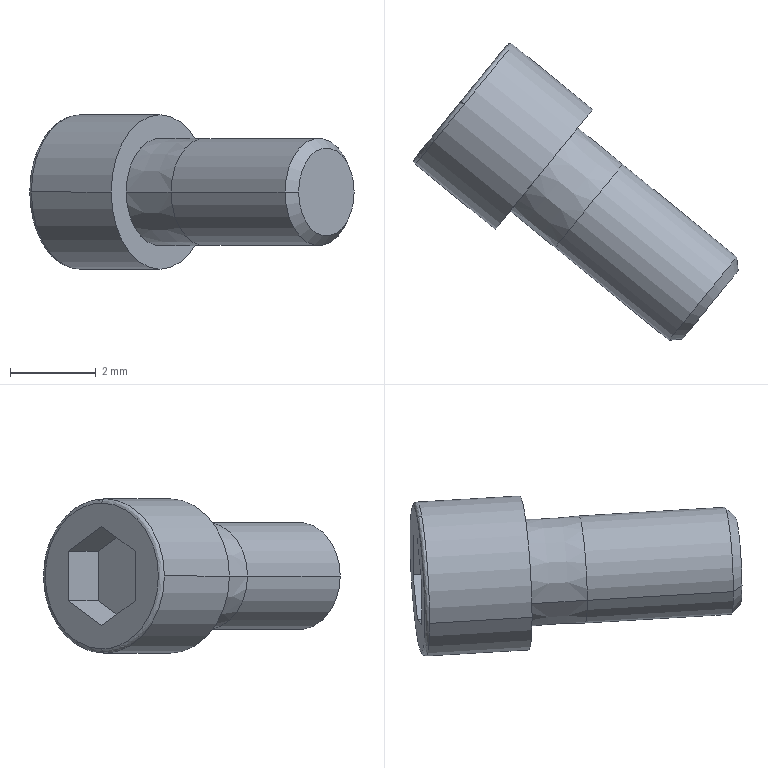Part | SolidWorks | features BaseBody 1 | 1 solid | 20 faces | box 7.56 x 6.916 x 3.6 mm | volume 45.965 mm3 | plane 10 | cylinder 4 | cone 4 | spline 2 | commonest cylinder face diameters 2.5 x2 3.6 x2
STEP:
#1=CARTESIAN_POINT('',(542.789,-161.255,300.245));
#2=VERTEX_POINT('',#1);
#3=CARTESIAN_POINT('',(543.924,-159.858,302.045));
#4=VERTEX_POINT('',#3);
#5=CARTESIAN_POINT('',(542.789,-161.255,302.045));
#6=DIRECTION('',(0.7758,-0.6309,-0.000000003));
#7=DIRECTION('',(0.6309,0.7758,0.));
#8=AXIS2_PLACEMENT_3D('',#5,#6,#7);
#9=CIRCLE('',#8,1.8);
#10=EDGE_CURVE('',#2,#4,#9,.T.);
#11=ORIENTED_EDGE('',*,*,#10,.F.);
#12=CARTESIAN_POINT('',(542.711,-161.191,300.345));
#13=VERTEX_POINT('',#12);
#14=CARTESIAN_POINT('',(542.789,-161.255,300.345));
#15=DIRECTION('',(0.6309,0.7758,0.000000002));
#16=DIRECTION('',(-0.000000001,0.000000003,-1.));
#17=AXIS2_PLACEMENT_3D('',#14,#15,#16);
#18=CIRCLE('',#17,0.1);
#19=EDGE_CURVE('',#2,#13,#18,.T.);
#20=ORIENTED_EDGE('',*,*,#19,.T.);
#21=CARTESIAN_POINT('',(542.711,-161.191,303.745));
#22=VERTEX_POINT('',#21);
#23=CARTESIAN_POINT('',(542.711,-161.191,300.345));
#24=CARTESIAN_POINT('',(544.856,-158.554,300.345));
#25=CARTESIAN_POINT('',(544.856,-158.554,303.745));
#26=CARTESIAN_POINT('',(542.711,-161.191,303.745));
#27=(BOUNDED_CURVE()B_SPLINE_CURVE(3,(#23,#24,#25,#26),.UNSPECIFIED.,.F.,.T.)B_SPLINE_CURVE_WITH_KNOTS((4,4),(0.,1.),.UNSPECIFIED.)CURVE()GEOMETRIC_REPRESENTATION_ITEM()RATIONAL_B_SPLINE_CURVE((1.,0.3333,0.3333,1.))REPRESENTATION_ITEM(''));
#28=EDGE_CURVE('',#13,#22,#27,.T.);
#29=ORIENTED_EDGE('',*,*,#28,.T.);
#30=CARTESIAN_POINT('',(542.789,-161.255,303.845));
#31=VERTEX_POINT('',#30);
#32=CARTESIAN_POINT('',(542.789,-161.255,303.745));
#33=DIRECTION('',(-0.6309,-0.7758,-0.000000002));
#34=DIRECTION('',(0.000000001,-0.000000003,1.));
#35=AXIS2_PLACEMENT_3D('',#32,#33,#34);
#36=CIRCLE('',#35,0.1);
#37=EDGE_CURVE('',#31,#22,#36,.T.);
#38=ORIENTED_EDGE('',*,*,#37,.F.);
#39=CARTESIAN_POINT('',(542.789,-161.255,302.045));
#40=DIRECTION('',(0.7758,-0.6309,-0.000000003));
#41=DIRECTION('',(0.6309,0.7758,0.));
#42=AXIS2_PLACEMENT_3D('',#39,#40,#41);
#43=CIRCLE('',#42,1.8);
#44=EDGE_CURVE('',#4,#31,#43,.T.);
#45=ORIENTED_EDGE('',*,*,#44,.F.);
#46=EDGE_LOOP('',(#11,#20,#29,#38,#45));
#47=FACE_OUTER_BOUND('',#46,.T.);
#48=CARTESIAN_POINT('',(542.789,-161.255,300.245));
#49=CARTESIAN_POINT('',(545.06,-158.462,300.245));
#50=CARTESIAN_POINT('',(545.06,-158.462,303.845));
#51=CARTESIAN_POINT('',(542.789,-161.255,303.845));
#52=CARTESIAN_POINT('',(542.743,-161.218,300.245));
#53=CARTESIAN_POINT('',(545.014,-158.425,300.245));
#54=CARTESIAN_POINT('',(545.014,-158.425,303.845));
#55=CARTESIAN_POINT('',(542.743,-161.218,303.845));
#56=CARTESIAN_POINT('',(542.711,-161.191,300.286));
#57=CARTESIAN_POINT('',(544.93,-158.463,300.286));
#58=CARTESIAN_POINT('',(544.93,-158.463,303.803));
#59=CARTESIAN_POINT('',(542.711,-161.191,303.803));
#60=CARTESIAN_POINT('',(542.711,-161.191,300.345));
#61=CARTESIAN_POINT('',(544.856,-158.554,300.345));
#62=CARTESIAN_POINT('',(544.856,-158.554,303.745));
#63=CARTESIAN_POINT('',(542.711,-161.191,303.745));
#64=(BOUNDED_SURFACE()B_SPLINE_SURFACE(3,3,((#48,#49,#50,#51),(#52,#53,#54,#55),(#56,#57,#58,#59),(#60,#61,#62,#63)),.UNSPECIFIED.,.F.,.F.,.T.)B_SPLINE_SURFACE_WITH_KNOTS((4,4),(4,4),(0.,1.),(0.,1.),.UNSPECIFIED.)GEOMETRIC_REPRESENTATION_ITEM()RATIONAL_B_SPLINE_SURFACE(((1.,0.3333,0.3333,1.),(0.8047,0.2682,0.2682,0.8047),(0.8047,0.2682,0.2682,0.8047),(1.,0.3333,0.3333,1.)))REPRESENTATION_ITEM('')SURFACE());
#65=ADVANCED_FACE('',(#47),#64,.T.);
#66=ORIENTED_EDGE('',*,*,#44,.T.);
#67=CARTESIAN_POINT('',(541.653,-162.651,302.045));
#68=VERTEX_POINT('',#67);
#69=CARTESIAN_POINT('',(542.789,-161.255,302.045));
#70=DIRECTION('',(0.7758,-0.6309,-0.000000003));
#71=DIRECTION('',(0.6309,0.7758,0.));
#72=AXIS2_PLACEMENT_3D('',#69,#70,#71);
#73=CIRCLE('',#72,1.8);
#74=EDGE_CURVE('',#31,#68,#73,.T.);
#75=ORIENTED_EDGE('',*,*,#74,.T.);
#76=CARTESIAN_POINT('',(543.515,-164.165,302.045));
#77=VERTEX_POINT('',#76);
#78=CARTESIAN_POINT('',(542.584,-163.408,302.045));
#79=DIRECTION('',(0.7758,-0.6309,-0.000000003));
#80=VECTOR('',#79,1000.);
#81=LINE('',#78,#80);
#82=EDGE_CURVE('',#68,#77,#81,.T.);
#83=ORIENTED_EDGE('',*,*,#82,.T.);
#84=CARTESIAN_POINT('',(545.786,-161.372,302.045));
#85=VERTEX_POINT('',#84);
#86=CARTESIAN_POINT('',(544.651,-162.769,302.045));
#87=DIRECTION('',(-0.7758,0.6309,0.000000003));
#88=DIRECTION('',(0.6309,0.7758,0.));
#89=AXIS2_PLACEMENT_3D('',#86,#87,#88);
#90=CIRCLE('',#89,1.8);
#91=EDGE_CURVE('',#77,#85,#90,.T.);
#92=ORIENTED_EDGE('',*,*,#91,.T.);
#93=CARTESIAN_POINT('',(544.855,-160.615,302.045));
#94=DIRECTION('',(0.7758,-0.6309,-0.000000003));
#95=VECTOR('',#94,1000.);
#96=LINE('',#93,#95);
#97=EDGE_CURVE('',#4,#85,#96,.T.);
#98=ORIENTED_EDGE('',*,*,#97,.F.);
#99=EDGE_LOOP('',(#66,#75,#83,#92,#98));
#100=FACE_OUTER_BOUND('',#99,.T.);
#101=CARTESIAN_POINT('',(543.72,-162.012,302.045));
#102=DIRECTION('',(0.7758,-0.6309,-0.000000003));
#103=DIRECTION('',(0.6309,0.7758,0.));
#104=AXIS2_PLACEMENT_3D('',#101,#102,#103);
#105=CYLINDRICAL_SURFACE('',#104,1.8);
#106=ADVANCED_FACE('',(#100),#105,.T.);
#107=CARTESIAN_POINT('',(543.862,-163.738,302.045));
#108=VERTEX_POINT('',#107);
#109=CARTESIAN_POINT('',(545.439,-161.799,302.045));
#110=VERTEX_POINT('',#109);
#111=CARTESIAN_POINT('',(544.651,-162.769,302.045));
#112=DIRECTION('',(-0.7758,0.6309,0.000000003));
#113=DIRECTION('',(0.6309,0.7758,0.));
#114=AXIS2_PLACEMENT_3D('',#111,#112,#113);
#115=CIRCLE('',#114,1.249);
#116=EDGE_CURVE('',#108,#110,#115,.T.);
#117=ORIENTED_EDGE('',*,*,#116,.F.);
#118=CARTESIAN_POINT('',(544.909,-164.59,302.045));
#119=VERTEX_POINT('',#118);
#120=CARTESIAN_POINT('',(544.909,-164.59,302.045));
#121=DIRECTION('',(0.7755,-0.6313,-0.000000003));
#122=VECTOR('',#121,1000.);
#123=LINE('',#120,#122);
#124=EDGE_CURVE('',#108,#119,#123,.T.);
#125=ORIENTED_EDGE('',*,*,#124,.T.);
#126=CARTESIAN_POINT('',(546.487,-162.651,302.045));
#127=VERTEX_POINT('',#126);
#128=CARTESIAN_POINT('',(545.698,-163.621,302.045));
#129=DIRECTION('',(-0.7758,0.6309,0.000000003));
#130=DIRECTION('',(0.000000001,-0.000000003,1.));
#131=AXIS2_PLACEMENT_3D('',#128,#129,#130);
#132=CIRCLE('',#131,1.25);
#133=EDGE_CURVE('',#119,#127,#132,.T.);
#134=ORIENTED_EDGE('',*,*,#133,.T.);
#135=CARTESIAN_POINT('',(546.487,-162.651,302.045));
#136=DIRECTION('',(0.7761,-0.6306,-0.000000003));
#137=VECTOR('',#136,1000.);
#138=LINE('',#135,#137);
#139=EDGE_CURVE('',#110,#127,#138,.T.);
#140=ORIENTED_EDGE('',*,*,#139,.F.);
#141=EDGE_LOOP('',(#117,#125,#134,#140));
#142=FACE_OUTER_BOUND('',#141,.T.);
#143=CARTESIAN_POINT('',(545.698,-163.621,302.045));
#144=DIRECTION('',(0.7758,-0.6309,-0.000000003));
#145=DIRECTION('',(0.6309,0.7758,0.));
#146=AXIS2_PLACEMENT_3D('',#143,#144,#145);
#147=CONICAL_SURFACE('',#146,1.25,0.000463);
#148=ADVANCED_FACE('',(#142),#147,.T.);
#149=ORIENTED_EDGE('',*,*,#133,.F.);
#150=CARTESIAN_POINT('',(547.567,-166.751,302.045));
#151=VERTEX_POINT('',#150);
#152=CARTESIAN_POINT('',(546.238,-165.671,302.045));
#153=DIRECTION('',(0.7758,-0.6309,-0.000000003));
#154=VECTOR('',#153,1000.);
#155=LINE('',#152,#154);
#156=EDGE_CURVE('',#119,#151,#155,.T.);
#157=ORIENTED_EDGE('',*,*,#156,.T.);
#158=CARTESIAN_POINT('',(549.144,-164.812,302.045));
#159=VERTEX_POINT('',#158);
#160=CARTESIAN_POINT('',(548.355,-165.781,302.045));
#161=DIRECTION('',(-0.7758,0.6309,0.000000003));
#162=DIRECTION('',(0.6309,0.7758,0.));
#163=AXIS2_PLACEMENT_3D('',#160,#161,#162);
#164=CIRCLE('',#163,1.25);
#165=EDGE_CURVE('',#151,#159,#164,.T.);
#166=ORIENTED_EDGE('',*,*,#165,.T.);
#167=CARTESIAN_POINT('',(547.815,-163.731,302.045));
#168=DIRECTION('',(0.7758,-0.6309,-0.000000003));
#169=VECTOR('',#168,1000.);
#170=LINE('',#167,#169);
#171=EDGE_CURVE('',#127,#159,#170,.T.);
#172=ORIENTED_EDGE('',*,*,#171,.F.);
#173=EDGE_LOOP('',(#149,#157,#166,#172));
#174=FACE_OUTER_BOUND('',#173,.T.);
#175=CARTESIAN_POINT('',(547.027,-164.701,302.045));
#176=DIRECTION('',(0.7758,-0.6309,-0.000000003));
#177=DIRECTION('',(0.6309,0.7758,0.));
#178=AXIS2_PLACEMENT_3D('',#175,#176,#177);
#179=CYLINDRICAL_SURFACE('',#178,1.25);
#180=ADVANCED_FACE('',(#174),#179,.T.);
#181=CARTESIAN_POINT('',(547.883,-166.719,302.045));
#182=VERTEX_POINT('',#181);
#183=CARTESIAN_POINT('',(549.176,-165.128,302.045));
#184=VERTEX_POINT('',#183);
#185=CARTESIAN_POINT('',(548.53,-165.923,302.045));
#186=DIRECTION('',(-0.7758,0.6309,0.000000003));
#187=DIRECTION('',(-0.6309,-0.7758,0.));
#188=AXIS2_PLACEMENT_3D('',#185,#186,#187);
#189=CIRCLE('',#188,1.025);
#190=EDGE_CURVE('',#182,#184,#189,.T.);
#191=ORIENTED_EDGE('',*,*,#190,.T.);
#192=CARTESIAN_POINT('',(549.144,-164.812,302.045));
#193=DIRECTION('',(-0.1025,0.9947,0.000000002));
#194=VECTOR('',#193,1000.);
#195=LINE('',#192,#194);
#196=EDGE_CURVE('',#184,#159,#195,.T.);
#197=ORIENTED_EDGE('',*,*,#196,.T.);
#198=ORIENTED_EDGE('',*,*,#165,.F.);
#199=CARTESIAN_POINT('',(547.567,-166.751,302.045));
#200=DIRECTION('',(-0.9947,-0.1025,0.000000002));
#201=VECTOR('',#200,1000.);
#202=LINE('',#199,#201);
#203=EDGE_CURVE('',#182,#151,#202,.T.);
#204=ORIENTED_EDGE('',*,*,#203,.F.);
#205=EDGE_LOOP('',(#191,#197,#198,#204));
#206=FACE_OUTER_BOUND('',#205,.T.);
#207=CARTESIAN_POINT('',(548.355,-165.781,302.045));
#208=DIRECTION('',(-0.7758,0.6309,0.000000003));
#209=DIRECTION('',(-0.6309,-0.7758,0.));
#210=AXIS2_PLACEMENT_3D('',#207,#208,#209);
#211=CONICAL_SURFACE('',#210,1.25,0.7854);
#212=ADVANCED_FACE('',(#206),#211,.T.);
#213=ORIENTED_EDGE('',*,*,#82,.F.);
#214=CARTESIAN_POINT('',(542.789,-161.255,302.045));
#215=DIRECTION('',(0.7758,-0.6309,-0.000000003));
#216=DIRECTION('',(0.6309,0.7758,0.));
#217=AXIS2_PLACEMENT_3D('',#214,#215,#216);
#218=CIRCLE('',#217,1.8);
#219=EDGE_CURVE('',#68,#2,#218,.T.);
#220=ORIENTED_EDGE('',*,*,#219,.T.);
#221=ORIENTED_EDGE('',*,*,#10,.T.);
#222=ORIENTED_EDGE('',*,*,#97,.T.);
#223=CARTESIAN_POINT('',(544.651,-162.769,302.045));
#224=DIRECTION('',(-0.7758,0.6309,0.000000003));
#225=DIRECTION('',(0.6309,0.7758,0.));
#226=AXIS2_PLACEMENT_3D('',#223,#224,#225);
#227=CIRCLE('',#226,1.8);
#228=EDGE_CURVE('',#85,#77,#227,.T.);
#229=ORIENTED_EDGE('',*,*,#228,.T.);
#230=EDGE_LOOP('',(#213,#220,#221,#222,#229));
#231=FACE_OUTER_BOUND('',#230,.T.);
#232=CARTESIAN_POINT('',(543.72,-162.012,302.045));
#233=DIRECTION('',(0.7758,-0.6309,-0.000000003));
#234=DIRECTION('',(0.6309,0.7758,0.));
#235=AXIS2_PLACEMENT_3D('',#232,#233,#234);
#236=CYLINDRICAL_SURFACE('',#235,1.8);
#237=ADVANCED_FACE('',(#231),#236,.T.);
#238=CARTESIAN_POINT('',(544.651,-162.769,302.045));
#239=DIRECTION('',(-0.7758,0.6309,0.000000003));
#240=DIRECTION('',(0.6309,0.7758,0.));
#241=AXIS2_PLACEMENT_3D('',#238,#239,#240);
#242=CIRCLE('',#241,1.249);
#243=EDGE_CURVE('',#110,#108,#242,.T.);
#244=ORIENTED_EDGE('',*,*,#243,.T.);
#245=ORIENTED_EDGE('',*,*,#116,.T.);
#246=EDGE_LOOP('',(#244,#245));
#247=FACE_BOUND('',#246,.T.);
#248=ORIENTED_EDGE('',*,*,#228,.F.);
#249=ORIENTED_EDGE('',*,*,#91,.F.);
#250=EDGE_LOOP('',(#248,#249));
#251=FACE_OUTER_BOUND('',#250,.T.);
#252=CARTESIAN_POINT('',(544.651,-162.769,302.945));
#253=DIRECTION('',(0.7758,-0.6309,-0.000000003));
#254=DIRECTION('',(0.6309,0.7758,0.));
#255=AXIS2_PLACEMENT_3D('',#252,#253,#254);
#256=PLANE('',#255);
#257=ADVANCED_FACE('',(#247,#251),#256,.T.);
#258=ORIENTED_EDGE('',*,*,#19,.F.);
#259=ORIENTED_EDGE('',*,*,#219,.F.);
#260=ORIENTED_EDGE('',*,*,#74,.F.);
#261=ORIENTED_EDGE('',*,*,#37,.T.);
#262=CARTESIAN_POINT('',(542.711,-161.191,303.745));
#263=CARTESIAN_POINT('',(540.566,-163.829,303.745));
#264=CARTESIAN_POINT('',(540.566,-163.829,300.345));
#265=CARTESIAN_POINT('',(542.711,-161.191,300.345));
#266=(BOUNDED_CURVE()B_SPLINE_CURVE(3,(#262,#263,#264,#265),.UNSPECIFIED.,.F.,.F.)B_SPLINE_CURVE_WITH_KNOTS((4,4),(0.,1.),.UNSPECIFIED.)CURVE()GEOMETRIC_REPRESENTATION_ITEM()RATIONAL_B_SPLINE_CURVE((1.,0.3333,0.3333,1.))REPRESENTATION_ITEM(''));
#267=EDGE_CURVE('',#22,#13,#266,.T.);
#268=ORIENTED_EDGE('',*,*,#267,.T.);
#269=EDGE_LOOP('',(#258,#259,#260,#261,#268));
#270=FACE_OUTER_BOUND('',#269,.T.);
#271=CARTESIAN_POINT('',(542.789,-161.255,303.845));
#272=CARTESIAN_POINT('',(540.517,-164.048,303.845));
#273=CARTESIAN_POINT('',(540.517,-164.048,300.245));
#274=CARTESIAN_POINT('',(542.789,-161.255,300.245));
#275=CARTESIAN_POINT('',(542.743,-161.218,303.845));
#276=CARTESIAN_POINT('',(540.472,-164.011,303.845));
#277=CARTESIAN_POINT('',(540.472,-164.011,300.245));
#278=CARTESIAN_POINT('',(542.743,-161.218,300.245));
#279=CARTESIAN_POINT('',(542.711,-161.191,303.803));
#280=CARTESIAN_POINT('',(540.492,-163.92,303.803));
#281=CARTESIAN_POINT('',(540.492,-163.92,300.286));
#282=CARTESIAN_POINT('',(542.711,-161.191,300.286));
#283=CARTESIAN_POINT('',(542.711,-161.191,303.745));
#284=CARTESIAN_POINT('',(540.566,-163.829,303.745));
#285=CARTESIAN_POINT('',(540.566,-163.829,300.345));
#286=CARTESIAN_POINT('',(542.711,-161.191,300.345));
#287=(BOUNDED_SURFACE()B_SPLINE_SURFACE(3,3,((#271,#272,#273,#274),(#275,#276,#277,#278),(#279,#280,#281,#282),(#283,#284,#285,#286)),.UNSPECIFIED.,.F.,.F.,.F.)B_SPLINE_SURFACE_WITH_KNOTS((4,4),(4,4),(0.,1.),(0.,1.),.UNSPECIFIED.)GEOMETRIC_REPRESENTATION_ITEM()RATIONAL_B_SPLINE_SURFACE(((1.,0.3333,0.3333,1.),(0.8047,0.2682,0.2682,0.8047),(0.8047,0.2682,0.2682,0.8047),(1.,0.3333,0.3333,1.)))REPRESENTATION_ITEM('')SURFACE());
#288=ADVANCED_FACE('',(#270),#287,.T.);
#289=ORIENTED_EDGE('',*,*,#124,.F.);
#290=ORIENTED_EDGE('',*,*,#243,.F.);
#291=ORIENTED_EDGE('',*,*,#139,.T.);
#292=CARTESIAN_POINT('',(545.698,-163.621,302.045));
#293=DIRECTION('',(-0.7758,0.6309,0.000000003));
#294=DIRECTION('',(0.000000001,-0.000000003,1.));
#295=AXIS2_PLACEMENT_3D('',#292,#293,#294);
#296=CIRCLE('',#295,1.25);
#297=EDGE_CURVE('',#127,#119,#296,.T.);
#298=ORIENTED_EDGE('',*,*,#297,.T.);
#299=EDGE_LOOP('',(#289,#290,#291,#298));
#300=FACE_OUTER_BOUND('',#299,.T.);
#301=CARTESIAN_POINT('',(545.698,-163.621,302.045));
#302=DIRECTION('',(0.7758,-0.6309,-0.000000003));
#303=DIRECTION('',(0.6309,0.7758,0.));
#304=AXIS2_PLACEMENT_3D('',#301,#302,#303);
#305=CONICAL_SURFACE('',#304,1.25,0.000463);
#306=ADVANCED_FACE('',(#300),#305,.T.);
#307=ORIENTED_EDGE('',*,*,#28,.F.);
#308=ORIENTED_EDGE('',*,*,#267,.F.);
#309=EDGE_LOOP('',(#307,#308));
#310=FACE_OUTER_BOUND('',#309,.T.);
#311=CARTESIAN_POINT('',(542.08,-161.967,301.467));
#312=VERTEX_POINT('',#311);
#313=CARTESIAN_POINT('',(542.711,-161.191,300.89));
#314=VERTEX_POINT('',#313);
#315=CARTESIAN_POINT('',(542.08,-161.967,301.467));
#316=DIRECTION('',(0.5464,0.6719,-0.5));
#317=VECTOR('',#316,1000.);
#318=LINE('',#315,#317);
#319=EDGE_CURVE('',#312,#314,#318,.T.);
#320=ORIENTED_EDGE('',*,*,#319,.T.);
#321=CARTESIAN_POINT('',(543.342,-160.416,301.467));
#322=VERTEX_POINT('',#321);
#323=CARTESIAN_POINT('',(542.711,-161.191,300.89));
#324=DIRECTION('',(0.5464,0.6719,0.5));
#325=VECTOR('',#324,1000.);
#326=LINE('',#323,#325);
#327=EDGE_CURVE('',#314,#322,#326,.T.);
#328=ORIENTED_EDGE('',*,*,#327,.T.);
#329=CARTESIAN_POINT('',(543.342,-160.416,302.622));
#330=VERTEX_POINT('',#329);
#331=CARTESIAN_POINT('',(543.342,-160.416,302.895));
#332=DIRECTION('',(0.000000002,-0.000000002,1.));
#333=VECTOR('',#332,1000.);
#334=LINE('',#331,#333);
#335=EDGE_CURVE('',#322,#330,#334,.T.);
#336=ORIENTED_EDGE('',*,*,#335,.T.);
#337=CARTESIAN_POINT('',(542.711,-161.191,303.199));
#338=VERTEX_POINT('',#337);
#339=CARTESIAN_POINT('',(543.342,-160.416,302.622));
#340=DIRECTION('',(-0.5464,-0.6719,0.5));
#341=VECTOR('',#340,1000.);
#342=LINE('',#339,#341);
#343=EDGE_CURVE('',#330,#338,#342,.T.);
#344=ORIENTED_EDGE('',*,*,#343,.T.);
#345=CARTESIAN_POINT('',(542.08,-161.967,302.622));
#346=VERTEX_POINT('',#345);
#347=CARTESIAN_POINT('',(542.711,-161.191,303.199));
#348=DIRECTION('',(-0.5464,-0.6719,-0.5));
#349=VECTOR('',#348,1000.);
#350=LINE('',#347,#349);
#351=EDGE_CURVE('',#338,#346,#350,.T.);
#352=ORIENTED_EDGE('',*,*,#351,.T.);
#353=CARTESIAN_POINT('',(542.08,-161.967,302.895));
#354=DIRECTION('',(-0.000000002,0.000000002,-1.));
#355=VECTOR('',#354,1000.);
#356=LINE('',#353,#355);
#357=EDGE_CURVE('',#346,#312,#356,.T.);
#358=ORIENTED_EDGE('',*,*,#357,.T.);
#359=EDGE_LOOP('',(#320,#328,#336,#344,#352,#358));
#360=FACE_BOUND('',#359,.T.);
#361=CARTESIAN_POINT('',(542.711,-161.191,302.895));
#362=DIRECTION('',(-0.7758,0.6309,0.000000003));
#363=DIRECTION('',(-0.6309,-0.7758,0.));
#364=AXIS2_PLACEMENT_3D('',#361,#362,#363);
#365=PLANE('',#364);
#366=ADVANCED_FACE('',(#310,#360),#365,.T.);
#367=ORIENTED_EDGE('',*,*,#156,.F.);
#368=ORIENTED_EDGE('',*,*,#297,.F.);
#369=ORIENTED_EDGE('',*,*,#171,.T.);
#370=CARTESIAN_POINT('',(548.355,-165.781,302.045));
#371=DIRECTION('',(-0.7758,0.6309,0.000000003));
#372=DIRECTION('',(0.6309,0.7758,0.));
#373=AXIS2_PLACEMENT_3D('',#370,#371,#372);
#374=CIRCLE('',#373,1.25);
#375=EDGE_CURVE('',#159,#151,#374,.T.);
#376=ORIENTED_EDGE('',*,*,#375,.T.);
#377=EDGE_LOOP('',(#367,#368,#369,#376));
#378=FACE_OUTER_BOUND('',#377,.T.);
#379=CARTESIAN_POINT('',(547.027,-164.701,302.045));
#380=DIRECTION('',(0.7758,-0.6309,-0.000000003));
#381=DIRECTION('',(0.6309,0.7758,0.));
#382=AXIS2_PLACEMENT_3D('',#379,#380,#381);
#383=CYLINDRICAL_SURFACE('',#382,1.25);
#384=ADVANCED_FACE('',(#378),#383,.T.);
#385=CARTESIAN_POINT('',(544.195,-161.11,301.467));
#386=VERTEX_POINT('',#385);
#387=CARTESIAN_POINT('',(543.342,-160.416,301.467));
#388=DIRECTION('',(0.7758,-0.6309,-0.000000003));
#389=VECTOR('',#388,1000.);
#390=LINE('',#387,#389);
#391=EDGE_CURVE('',#322,#386,#390,.T.);
#392=ORIENTED_EDGE('',*,*,#391,.F.);
#393=ORIENTED_EDGE('',*,*,#327,.F.);
#394=CARTESIAN_POINT('',(543.564,-161.886,300.89));
#395=VERTEX_POINT('',#394);
#396=CARTESIAN_POINT('',(543.564,-161.886,300.89));
#397=DIRECTION('',(-0.7758,0.6309,0.000000003));
#398=VECTOR('',#397,1000.);
#399=LINE('',#396,#398);
#400=EDGE_CURVE('',#395,#314,#399,.T.);
#401=ORIENTED_EDGE('',*,*,#400,.F.);
#402=CARTESIAN_POINT('',(544.195,-161.11,301.467));
#403=DIRECTION('',(-0.5464,-0.6719,-0.5));
#404=VECTOR('',#403,1000.);
#405=LINE('',#402,#404);
#406=EDGE_CURVE('',#386,#395,#405,.T.);
#407=ORIENTED_EDGE('',*,*,#406,.F.);
#408=EDGE_LOOP('',(#392,#393,#401,#407));
#409=FACE_OUTER_BOUND('',#408,.T.);
#410=CARTESIAN_POINT('',(543.342,-160.416,301.467));
#411=DIRECTION('',(0.3155,0.3879,-0.866));
#412=DIRECTION('',(0.,0.9126,0.4088));
#413=AXIS2_PLACEMENT_3D('',#410,#411,#412);
#414=PLANE('',#413);
#415=ADVANCED_FACE('',(#409),#414,.F.);
#416=ORIENTED_EDGE('',*,*,#400,.T.);
#417=ORIENTED_EDGE('',*,*,#319,.F.);
#418=CARTESIAN_POINT('',(542.933,-162.661,301.467));
#419=VERTEX_POINT('',#418);
#420=CARTESIAN_POINT('',(542.933,-162.661,301.467));
#421=DIRECTION('',(-0.7758,0.6309,0.000000003));
#422=VECTOR('',#421,1000.);
#423=LINE('',#420,#422);
#424=EDGE_CURVE('',#419,#312,#423,.T.);
#425=ORIENTED_EDGE('',*,*,#424,.F.);
#426=CARTESIAN_POINT('',(543.564,-161.886,300.89));
#427=DIRECTION('',(-0.5464,-0.6719,0.5));
#428=VECTOR('',#427,1000.);
#429=LINE('',#426,#428);
#430=EDGE_CURVE('',#395,#419,#429,.T.);
#431=ORIENTED_EDGE('',*,*,#430,.F.);
#432=EDGE_LOOP('',(#416,#417,#425,#431));
#433=FACE_OUTER_BOUND('',#432,.T.);
#434=CARTESIAN_POINT('',(542.711,-161.191,300.89));
#435=DIRECTION('',(-0.3155,-0.3879,-0.866));
#436=DIRECTION('',(0.,0.9126,-0.4088));
#437=AXIS2_PLACEMENT_3D('',#434,#435,#436);
#438=PLANE('',#437);
#439=ADVANCED_FACE('',(#433),#438,.F.);
#440=ORIENTED_EDGE('',*,*,#424,.T.);
#441=ORIENTED_EDGE('',*,*,#357,.F.);
#442=CARTESIAN_POINT('',(542.933,-162.661,302.622));
#443=VERTEX_POINT('',#442);
#444=CARTESIAN_POINT('',(542.08,-161.967,302.622));
#445=DIRECTION('',(-0.7758,0.6309,0.));
#446=VECTOR('',#445,1000.);
#447=LINE('',#444,#446);
#448=EDGE_CURVE('',#443,#346,#447,.T.);
#449=ORIENTED_EDGE('',*,*,#448,.F.);
#450=CARTESIAN_POINT('',(542.933,-162.661,301.467));
#451=DIRECTION('',(-0.000000001,-0.000000002,1.));
#452=VECTOR('',#451,1000.);
#453=LINE('',#450,#452);
#454=EDGE_CURVE('',#419,#443,#453,.T.);
#455=ORIENTED_EDGE('',*,*,#454,.F.);
#456=EDGE_LOOP('',(#440,#441,#449,#455));
#457=FACE_OUTER_BOUND('',#456,.T.);
#458=CARTESIAN_POINT('',(542.08,-161.967,301.467));
#459=DIRECTION('',(-0.6309,-0.7758,-0.000000002));
#460=DIRECTION('',(0.7758,-0.6309,0.));
#461=AXIS2_PLACEMENT_3D('',#458,#459,#460);
#462=PLANE('',#461);
#463=ADVANCED_FACE('',(#457),#462,.F.);
#464=ORIENTED_EDGE('',*,*,#448,.T.);
#465=ORIENTED_EDGE('',*,*,#351,.F.);
#466=CARTESIAN_POINT('',(543.564,-161.886,303.199));
#467=VERTEX_POINT('',#466);
#468=CARTESIAN_POINT('',(543.564,-161.886,303.199));
#469=DIRECTION('',(-0.7758,0.6309,0.000000003));
#470=VECTOR('',#469,1000.);
#471=LINE('',#468,#470);
#472=EDGE_CURVE('',#467,#338,#471,.T.);
#473=ORIENTED_EDGE('',*,*,#472,.F.);
#474=CARTESIAN_POINT('',(542.933,-162.661,302.622));
#475=DIRECTION('',(0.5464,0.6719,0.5));
#476=VECTOR('',#475,1000.);
#477=LINE('',#474,#476);
#478=EDGE_CURVE('',#443,#467,#477,.T.);
#479=ORIENTED_EDGE('',*,*,#478,.F.);
#480=EDGE_LOOP('',(#464,#465,#473,#479));
#481=FACE_OUTER_BOUND('',#480,.T.);
#482=CARTESIAN_POINT('',(542.08,-161.967,302.622));
#483=DIRECTION('',(-0.3155,-0.3879,0.866));
#484=DIRECTION('',(0.,-0.9126,-0.4088));
#485=AXIS2_PLACEMENT_3D('',#482,#483,#484);
#486=PLANE('',#485);
#487=ADVANCED_FACE('',(#481),#486,.F.);
#488=ORIENTED_EDGE('',*,*,#472,.T.);
#489=ORIENTED_EDGE('',*,*,#343,.F.);
#490=CARTESIAN_POINT('',(544.195,-161.11,302.622));
#491=VERTEX_POINT('',#490);
#492=CARTESIAN_POINT('',(544.195,-161.11,302.622));
#493=DIRECTION('',(-0.7758,0.6309,0.000000003));
#494=VECTOR('',#493,1000.);
#495=LINE('',#492,#494);
#496=EDGE_CURVE('',#491,#330,#495,.T.);
#497=ORIENTED_EDGE('',*,*,#496,.F.);
#498=CARTESIAN_POINT('',(543.564,-161.886,303.199));
#499=DIRECTION('',(0.5464,0.6719,-0.5));
#500=VECTOR('',#499,1000.);
#501=LINE('',#498,#500);
#502=EDGE_CURVE('',#467,#491,#501,.T.);
#503=ORIENTED_EDGE('',*,*,#502,.F.);
#504=EDGE_LOOP('',(#488,#489,#497,#503));
#505=FACE_OUTER_BOUND('',#504,.T.);
#506=CARTESIAN_POINT('',(542.711,-161.191,303.199));
#507=DIRECTION('',(0.3155,0.3879,0.866));
#508=DIRECTION('',(0.,-0.9126,0.4088));
#509=AXIS2_PLACEMENT_3D('',#506,#507,#508);
#510=PLANE('',#509);
#511=ADVANCED_FACE('',(#505),#510,.F.);
#512=ORIENTED_EDGE('',*,*,#496,.T.);
#513=ORIENTED_EDGE('',*,*,#335,.F.);
#514=ORIENTED_EDGE('',*,*,#391,.T.);
#515=CARTESIAN_POINT('',(544.195,-161.11,302.622));
#516=DIRECTION('',(0.000000001,0.000000002,-1.));
#517=VECTOR('',#516,1000.);
#518=LINE('',#515,#517);
#519=EDGE_CURVE('',#491,#386,#518,.T.);
#520=ORIENTED_EDGE('',*,*,#519,.F.);
#521=EDGE_LOOP('',(#512,#513,#514,#520));
#522=FACE_OUTER_BOUND('',#521,.T.);
#523=CARTESIAN_POINT('',(543.342,-160.416,302.622));
#524=DIRECTION('',(0.6309,0.7758,0.000000002));
#525=DIRECTION('',(-0.7758,0.6309,0.));
#526=AXIS2_PLACEMENT_3D('',#523,#524,#525);
#527=PLANE('',#526);
#528=ADVANCED_FACE('',(#522),#527,.F.);
#529=ORIENTED_EDGE('',*,*,#196,.F.);
#530=CARTESIAN_POINT('',(548.53,-165.923,302.045));
#531=DIRECTION('',(-0.7758,0.6309,0.000000003));
#532=DIRECTION('',(-0.6309,-0.7758,0.));
#533=AXIS2_PLACEMENT_3D('',#530,#531,#532);
#534=CIRCLE('',#533,1.025);
#535=EDGE_CURVE('',#184,#182,#534,.T.);
#536=ORIENTED_EDGE('',*,*,#535,.T.);
#537=ORIENTED_EDGE('',*,*,#203,.T.);
#538=ORIENTED_EDGE('',*,*,#375,.F.);
#539=EDGE_LOOP('',(#529,#536,#537,#538));
#540=FACE_OUTER_BOUND('',#539,.T.);
#541=CARTESIAN_POINT('',(548.355,-165.781,302.045));
#542=DIRECTION('',(-0.7758,0.6309,0.000000003));
#543=DIRECTION('',(-0.6309,-0.7758,0.));
#544=AXIS2_PLACEMENT_3D('',#541,#542,#543);
#545=CONICAL_SURFACE('',#544,1.25,0.7854);
#546=ADVANCED_FACE('',(#540),#545,.T.);
#547=ORIENTED_EDGE('',*,*,#478,.T.);
#548=ORIENTED_EDGE('',*,*,#502,.T.);
#549=ORIENTED_EDGE('',*,*,#519,.T.);
#550=ORIENTED_EDGE('',*,*,#406,.T.);
#551=ORIENTED_EDGE('',*,*,#430,.T.);
#552=ORIENTED_EDGE('',*,*,#454,.T.);
#553=EDGE_LOOP('',(#547,#548,#549,#550,#551,#552));
#554=FACE_OUTER_BOUND('',#553,.T.);
#555=CARTESIAN_POINT('',(543.564,-161.886,302.045));
#556=DIRECTION('',(-0.7758,0.6309,0.000000003));
#557=DIRECTION('',(-0.6309,-0.7758,0.));
#558=AXIS2_PLACEMENT_3D('',#555,#556,#557);
#559=PLANE('',#558);
#560=ADVANCED_FACE('',(#554),#559,.T.);
#561=ORIENTED_EDGE('',*,*,#190,.F.);
#562=ORIENTED_EDGE('',*,*,#535,.F.);
#563=EDGE_LOOP('',(#561,#562));
#564=FACE_OUTER_BOUND('',#563,.T.);
#565=CARTESIAN_POINT('',(548.53,-165.923,302.557));
#566=DIRECTION('',(0.7758,-0.6309,-0.000000003));
#567=DIRECTION('',(0.6309,0.7758,0.));
#568=AXIS2_PLACEMENT_3D('',#565,#566,#567);
#569=PLANE('',#568);
#570=ADVANCED_FACE('',(#564),#569,.T.);
#571=CLOSED_SHELL('',(#65,#106,#148,#180,#212,#237,#257,#288,#306,#366,#384,#415,#439,#463,#487,#511,#528,#546,#560,#570));
#572=MANIFOLD_SOLID_BREP('',#571);
#573=CARTESIAN_POINT('',(0.,0.,0.));
#574=DIRECTION('',(0.,0.,1.));
#575=DIRECTION('',(1.,0.,0.));
#576=AXIS2_PLACEMENT_3D('',#573,#574,#575);
#577=(LENGTH_UNIT()NAMED_UNIT(*)SI_UNIT(.MILLI.,.METRE.));
#578=UNCERTAINTY_MEASURE_WITH_UNIT(LENGTH_MEASURE(0.00001),#577,'','');
#579=(NAMED_UNIT(*)PLANE_ANGLE_UNIT()SI_UNIT($,.RADIAN.));
#580=(NAMED_UNIT(*)SI_UNIT($,.STERADIAN.)SOLID_ANGLE_UNIT());
#581=(GEOMETRIC_REPRESENTATION_CONTEXT(3)GLOBAL_UNCERTAINTY_ASSIGNED_CONTEXT((#578))GLOBAL_UNIT_ASSIGNED_CONTEXT((#577,#579,#580))REPRESENTATION_CONTEXT('',''));
#582=ADVANCED_BREP_SHAPE_REPRESENTATION('',(#572,#576),#581);